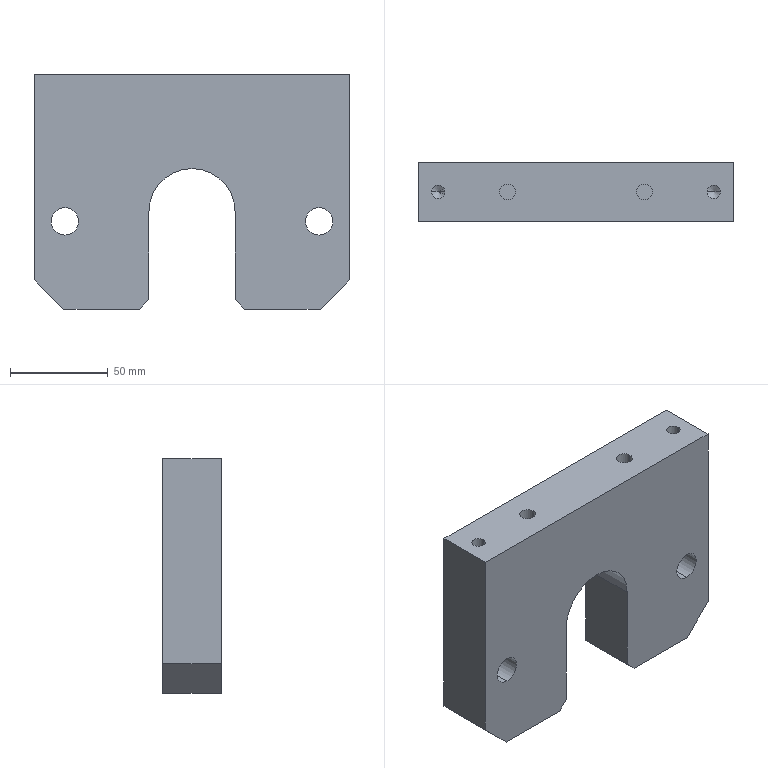Part | SolidWorks | features Chamfer 2, HoleWzd 2, ICE 2, Extrusion 1 | 1 solid | 33 faces | box 161 x 30 x 120 mm | volume 471064 mm3 | plane 15 | cylinder 14 | cone 4 | commonest cylinder face diameters 6.8 x4 8 x4 14 x4 44 x2
STEP:
#1=CARTESIAN_POINT('',(31.,15.,45.));
#2=VERTEX_POINT('',#1);
#3=CARTESIAN_POINT('',(39.,15.,45.));
#4=VERTEX_POINT('',#3);
#5=CARTESIAN_POINT('',(35.,15.,45.));
#6=DIRECTION('',(0.,0.,1.));
#7=DIRECTION('',(1.,0.,0.));
#8=AXIS2_PLACEMENT_3D('',#5,#6,#7);
#9=CIRCLE('',#8,4.);
#10=EDGE_CURVE('',#2,#4,#9,.T.);
#11=ORIENTED_EDGE('',*,*,#10,.F.);
#12=CARTESIAN_POINT('',(31.,15.,60.));
#13=VERTEX_POINT('',#12);
#14=CARTESIAN_POINT('',(31.,15.,45.));
#15=DIRECTION('',(0.,0.,1.));
#16=VECTOR('',#15,1000.);
#17=LINE('',#14,#16);
#18=EDGE_CURVE('',#2,#13,#17,.T.);
#19=ORIENTED_EDGE('',*,*,#18,.T.);
#20=CARTESIAN_POINT('',(39.,15.,60.));
#21=VERTEX_POINT('',#20);
#22=CARTESIAN_POINT('',(35.,15.,60.));
#23=DIRECTION('',(0.,0.,1.));
#24=DIRECTION('',(1.,0.,0.));
#25=AXIS2_PLACEMENT_3D('',#22,#23,#24);
#26=CIRCLE('',#25,4.);
#27=EDGE_CURVE('',#13,#21,#26,.T.);
#28=ORIENTED_EDGE('',*,*,#27,.T.);
#29=CARTESIAN_POINT('',(39.,15.,45.));
#30=DIRECTION('',(0.,0.,1.));
#31=VECTOR('',#30,1000.);
#32=LINE('',#29,#31);
#33=EDGE_CURVE('',#4,#21,#32,.T.);
#34=ORIENTED_EDGE('',*,*,#33,.F.);
#35=EDGE_LOOP('',(#11,#19,#28,#34));
#36=FACE_OUTER_BOUND('',#35,.T.);
#37=CARTESIAN_POINT('',(35.,15.,45.));
#38=DIRECTION('',(0.,0.,1.));
#39=DIRECTION('',(1.,0.,0.));
#40=AXIS2_PLACEMENT_3D('',#37,#38,#39);
#41=CYLINDRICAL_SURFACE('',#40,4.);
#42=ADVANCED_FACE('',(#36),#41,.F.);
#43=CARTESIAN_POINT('',(-39.,15.,45.));
#44=VERTEX_POINT('',#43);
#45=CARTESIAN_POINT('',(-31.,15.,45.));
#46=VERTEX_POINT('',#45);
#47=CARTESIAN_POINT('',(-35.,15.,45.));
#48=DIRECTION('',(0.,0.,1.));
#49=DIRECTION('',(1.,0.,0.));
#50=AXIS2_PLACEMENT_3D('',#47,#48,#49);
#51=CIRCLE('',#50,4.);
#52=EDGE_CURVE('',#44,#46,#51,.T.);
#53=ORIENTED_EDGE('',*,*,#52,.F.);
#54=CARTESIAN_POINT('',(-39.,15.,60.));
#55=VERTEX_POINT('',#54);
#56=CARTESIAN_POINT('',(-39.,15.,45.));
#57=DIRECTION('',(0.,0.,1.));
#58=VECTOR('',#57,1000.);
#59=LINE('',#56,#58);
#60=EDGE_CURVE('',#44,#55,#59,.T.);
#61=ORIENTED_EDGE('',*,*,#60,.T.);
#62=CARTESIAN_POINT('',(-31.,15.,60.));
#63=VERTEX_POINT('',#62);
#64=CARTESIAN_POINT('',(-35.,15.,60.));
#65=DIRECTION('',(0.,0.,1.));
#66=DIRECTION('',(1.,0.,0.));
#67=AXIS2_PLACEMENT_3D('',#64,#65,#66);
#68=CIRCLE('',#67,4.);
#69=EDGE_CURVE('',#55,#63,#68,.T.);
#70=ORIENTED_EDGE('',*,*,#69,.T.);
#71=CARTESIAN_POINT('',(-31.,15.,45.));
#72=DIRECTION('',(0.,0.,1.));
#73=VECTOR('',#72,1000.);
#74=LINE('',#71,#73);
#75=EDGE_CURVE('',#46,#63,#74,.T.);
#76=ORIENTED_EDGE('',*,*,#75,.F.);
#77=EDGE_LOOP('',(#53,#61,#70,#76));
#78=FACE_OUTER_BOUND('',#77,.T.);
#79=CARTESIAN_POINT('',(-35.,15.,45.));
#80=DIRECTION('',(0.,0.,1.));
#81=DIRECTION('',(1.,0.,0.));
#82=AXIS2_PLACEMENT_3D('',#79,#80,#81);
#83=CYLINDRICAL_SURFACE('',#82,4.);
#84=ADVANCED_FACE('',(#78),#83,.F.);
#85=CARTESIAN_POINT('',(67.1,15.,40.25));
#86=VERTEX_POINT('',#85);
#87=CARTESIAN_POINT('',(73.9,15.,40.25));
#88=VERTEX_POINT('',#87);
#89=CARTESIAN_POINT('',(70.5,15.,40.25));
#90=DIRECTION('',(0.,0.,1.));
#91=DIRECTION('',(1.,0.,0.));
#92=AXIS2_PLACEMENT_3D('',#89,#90,#91);
#93=CIRCLE('',#92,3.4);
#94=EDGE_CURVE('',#86,#88,#93,.T.);
#95=ORIENTED_EDGE('',*,*,#94,.F.);
#96=CARTESIAN_POINT('',(67.1,15.,60.));
#97=VERTEX_POINT('',#96);
#98=CARTESIAN_POINT('',(67.1,15.,60.));
#99=DIRECTION('',(0.,0.,1.));
#100=VECTOR('',#99,1000.);
#101=LINE('',#98,#100);
#102=EDGE_CURVE('',#86,#97,#101,.T.);
#103=ORIENTED_EDGE('',*,*,#102,.T.);
#104=CARTESIAN_POINT('',(73.9,15.,60.));
#105=VERTEX_POINT('',#104);
#106=CARTESIAN_POINT('',(70.5,15.,60.));
#107=DIRECTION('',(0.,0.,1.));
#108=DIRECTION('',(1.,0.,0.));
#109=AXIS2_PLACEMENT_3D('',#106,#107,#108);
#110=CIRCLE('',#109,3.4);
#111=EDGE_CURVE('',#97,#105,#110,.T.);
#112=ORIENTED_EDGE('',*,*,#111,.T.);
#113=CARTESIAN_POINT('',(73.9,15.,60.));
#114=DIRECTION('',(0.,0.,1.));
#115=VECTOR('',#114,1000.);
#116=LINE('',#113,#115);
#117=EDGE_CURVE('',#88,#105,#116,.T.);
#118=ORIENTED_EDGE('',*,*,#117,.F.);
#119=EDGE_LOOP('',(#95,#103,#112,#118));
#120=FACE_OUTER_BOUND('',#119,.T.);
#121=CARTESIAN_POINT('',(70.5,15.,60.));
#122=DIRECTION('',(0.,0.,1.));
#123=DIRECTION('',(1.,0.,0.));
#124=AXIS2_PLACEMENT_3D('',#121,#122,#123);
#125=CYLINDRICAL_SURFACE('',#124,3.4);
#126=ADVANCED_FACE('',(#120),#125,.F.);
#127=CARTESIAN_POINT('',(70.5,15.,38.207));
#128=VERTEX_POINT('',#127);
#129=CARTESIAN_POINT('',(73.9,15.,40.25));
#130=DIRECTION('',(0.8572,0.,0.515));
#131=VECTOR('',#130,1000.);
#132=LINE('',#129,#131);
#133=EDGE_CURVE('',#128,#88,#132,.T.);
#134=ORIENTED_EDGE('',*,*,#133,.F.);
#135=CARTESIAN_POINT('',(67.1,15.,40.25));
#136=DIRECTION('',(-0.8572,0.,0.515));
#137=VECTOR('',#136,1000.);
#138=LINE('',#135,#137);
#139=EDGE_CURVE('',#128,#86,#138,.T.);
#140=ORIENTED_EDGE('',*,*,#139,.T.);
#141=ORIENTED_EDGE('',*,*,#94,.T.);
#142=EDGE_LOOP('',(#134,#140,#141));
#143=FACE_OUTER_BOUND('',#142,.T.);
#144=CARTESIAN_POINT('',(70.5,15.,40.25));
#145=DIRECTION('',(0.,0.,1.));
#146=DIRECTION('',(1.,0.,0.));
#147=AXIS2_PLACEMENT_3D('',#144,#145,#146);
#148=CONICAL_SURFACE('',#147,3.4,1.03);
#149=ADVANCED_FACE('',(#143),#148,.F.);
#150=CARTESIAN_POINT('',(-73.9,15.,40.25));
#151=VERTEX_POINT('',#150);
#152=CARTESIAN_POINT('',(-67.1,15.,40.25));
#153=VERTEX_POINT('',#152);
#154=CARTESIAN_POINT('',(-70.5,15.,40.25));
#155=DIRECTION('',(0.,0.,1.));
#156=DIRECTION('',(1.,0.,0.));
#157=AXIS2_PLACEMENT_3D('',#154,#155,#156);
#158=CIRCLE('',#157,3.4);
#159=EDGE_CURVE('',#151,#153,#158,.T.);
#160=ORIENTED_EDGE('',*,*,#159,.F.);
#161=CARTESIAN_POINT('',(-73.9,15.,60.));
#162=VERTEX_POINT('',#161);
#163=CARTESIAN_POINT('',(-73.9,15.,60.));
#164=DIRECTION('',(0.,0.,1.));
#165=VECTOR('',#164,1000.);
#166=LINE('',#163,#165);
#167=EDGE_CURVE('',#151,#162,#166,.T.);
#168=ORIENTED_EDGE('',*,*,#167,.T.);
#169=CARTESIAN_POINT('',(-67.1,15.,60.));
#170=VERTEX_POINT('',#169);
#171=CARTESIAN_POINT('',(-70.5,15.,60.));
#172=DIRECTION('',(0.,0.,1.));
#173=DIRECTION('',(1.,0.,0.));
#174=AXIS2_PLACEMENT_3D('',#171,#172,#173);
#175=CIRCLE('',#174,3.4);
#176=EDGE_CURVE('',#162,#170,#175,.T.);
#177=ORIENTED_EDGE('',*,*,#176,.T.);
#178=CARTESIAN_POINT('',(-67.1,15.,60.));
#179=DIRECTION('',(0.,0.,1.));
#180=VECTOR('',#179,1000.);
#181=LINE('',#178,#180);
#182=EDGE_CURVE('',#153,#170,#181,.T.);
#183=ORIENTED_EDGE('',*,*,#182,.F.);
#184=EDGE_LOOP('',(#160,#168,#177,#183));
#185=FACE_OUTER_BOUND('',#184,.T.);
#186=CARTESIAN_POINT('',(-70.5,15.,60.));
#187=DIRECTION('',(0.,0.,1.));
#188=DIRECTION('',(1.,0.,0.));
#189=AXIS2_PLACEMENT_3D('',#186,#187,#188);
#190=CYLINDRICAL_SURFACE('',#189,3.4);
#191=ADVANCED_FACE('',(#185),#190,.F.);
#192=CARTESIAN_POINT('',(-70.5,15.,38.207));
#193=VERTEX_POINT('',#192);
#194=CARTESIAN_POINT('',(-67.1,15.,40.25));
#195=DIRECTION('',(0.8572,0.,0.515));
#196=VECTOR('',#195,1000.);
#197=LINE('',#194,#196);
#198=EDGE_CURVE('',#193,#153,#197,.T.);
#199=ORIENTED_EDGE('',*,*,#198,.F.);
#200=CARTESIAN_POINT('',(-73.9,15.,40.25));
#201=DIRECTION('',(-0.8572,0.,0.515));
#202=VECTOR('',#201,1000.);
#203=LINE('',#200,#202);
#204=EDGE_CURVE('',#193,#151,#203,.T.);
#205=ORIENTED_EDGE('',*,*,#204,.T.);
#206=ORIENTED_EDGE('',*,*,#159,.T.);
#207=EDGE_LOOP('',(#199,#205,#206));
#208=FACE_OUTER_BOUND('',#207,.T.);
#209=CARTESIAN_POINT('',(-70.5,15.,40.25));
#210=DIRECTION('',(0.,0.,1.));
#211=DIRECTION('',(1.,0.,0.));
#212=AXIS2_PLACEMENT_3D('',#209,#210,#211);
#213=CONICAL_SURFACE('',#212,3.4,1.03);
#214=ADVANCED_FACE('',(#208),#213,.F.);
#215=CARTESIAN_POINT('',(-65.,0.,-22.));
#216=VERTEX_POINT('',#215);
#217=CARTESIAN_POINT('',(-65.,0.,-8.));
#218=VERTEX_POINT('',#217);
#219=CARTESIAN_POINT('',(-65.,0.,-15.));
#220=DIRECTION('',(0.,1.,0.));
#221=DIRECTION('',(0.,0.,1.));
#222=AXIS2_PLACEMENT_3D('',#219,#220,#221);
#223=CIRCLE('',#222,7.);
#224=EDGE_CURVE('',#216,#218,#223,.T.);
#225=ORIENTED_EDGE('',*,*,#224,.F.);
#226=CARTESIAN_POINT('',(-65.,30.,-22.));
#227=VERTEX_POINT('',#226);
#228=CARTESIAN_POINT('',(-65.,30.,-22.));
#229=DIRECTION('',(0.,1.,0.));
#230=VECTOR('',#229,1000.);
#231=LINE('',#228,#230);
#232=EDGE_CURVE('',#216,#227,#231,.T.);
#233=ORIENTED_EDGE('',*,*,#232,.T.);
#234=CARTESIAN_POINT('',(-65.,30.,-8.));
#235=VERTEX_POINT('',#234);
#236=CARTESIAN_POINT('',(-65.,30.,-15.));
#237=DIRECTION('',(0.,1.,0.));
#238=DIRECTION('',(0.,0.,1.));
#239=AXIS2_PLACEMENT_3D('',#236,#237,#238);
#240=CIRCLE('',#239,7.);
#241=EDGE_CURVE('',#227,#235,#240,.T.);
#242=ORIENTED_EDGE('',*,*,#241,.T.);
#243=CARTESIAN_POINT('',(-65.,30.,-8.));
#244=DIRECTION('',(0.,1.,0.));
#245=VECTOR('',#244,1000.);
#246=LINE('',#243,#245);
#247=EDGE_CURVE('',#218,#235,#246,.T.);
#248=ORIENTED_EDGE('',*,*,#247,.F.);
#249=EDGE_LOOP('',(#225,#233,#242,#248));
#250=FACE_OUTER_BOUND('',#249,.T.);
#251=CARTESIAN_POINT('',(-65.,30.,-15.));
#252=DIRECTION('',(0.,1.,0.));
#253=DIRECTION('',(0.,0.,1.));
#254=AXIS2_PLACEMENT_3D('',#251,#252,#253);
#255=CYLINDRICAL_SURFACE('',#254,7.);
#256=ADVANCED_FACE('',(#250),#255,.F.);
#257=CARTESIAN_POINT('',(65.,0.,-22.));
#258=VERTEX_POINT('',#257);
#259=CARTESIAN_POINT('',(65.,0.,-8.));
#260=VERTEX_POINT('',#259);
#261=CARTESIAN_POINT('',(65.,0.,-15.));
#262=DIRECTION('',(0.,1.,0.));
#263=DIRECTION('',(0.,0.,1.));
#264=AXIS2_PLACEMENT_3D('',#261,#262,#263);
#265=CIRCLE('',#264,7.);
#266=EDGE_CURVE('',#258,#260,#265,.T.);
#267=ORIENTED_EDGE('',*,*,#266,.F.);
#268=CARTESIAN_POINT('',(65.,30.,-22.));
#269=VERTEX_POINT('',#268);
#270=CARTESIAN_POINT('',(65.,30.,-22.));
#271=DIRECTION('',(0.,1.,0.));
#272=VECTOR('',#271,1000.);
#273=LINE('',#270,#272);
#274=EDGE_CURVE('',#258,#269,#273,.T.);
#275=ORIENTED_EDGE('',*,*,#274,.T.);
#276=CARTESIAN_POINT('',(65.,30.,-8.));
#277=VERTEX_POINT('',#276);
#278=CARTESIAN_POINT('',(65.,30.,-15.));
#279=DIRECTION('',(0.,1.,0.));
#280=DIRECTION('',(0.,0.,1.));
#281=AXIS2_PLACEMENT_3D('',#278,#279,#280);
#282=CIRCLE('',#281,7.);
#283=EDGE_CURVE('',#269,#277,#282,.T.);
#284=ORIENTED_EDGE('',*,*,#283,.T.);
#285=CARTESIAN_POINT('',(65.,30.,-8.));
#286=DIRECTION('',(0.,1.,0.));
#287=VECTOR('',#286,1000.);
#288=LINE('',#285,#287);
#289=EDGE_CURVE('',#260,#277,#288,.T.);
#290=ORIENTED_EDGE('',*,*,#289,.F.);
#291=EDGE_LOOP('',(#267,#275,#284,#290));
#292=FACE_OUTER_BOUND('',#291,.T.);
#293=CARTESIAN_POINT('',(65.,30.,-15.));
#294=DIRECTION('',(0.,1.,0.));
#295=DIRECTION('',(0.,0.,1.));
#296=AXIS2_PLACEMENT_3D('',#293,#294,#295);
#297=CYLINDRICAL_SURFACE('',#296,7.);
#298=ADVANCED_FACE('',(#292),#297,.F.);
#299=CARTESIAN_POINT('',(0.,0.,12.));
#300=VERTEX_POINT('',#299);
#301=CARTESIAN_POINT('',(22.,0.,-10.));
#302=VERTEX_POINT('',#301);
#303=CARTESIAN_POINT('',(0.,0.,-10.));
#304=DIRECTION('',(0.,1.,0.));
#305=DIRECTION('',(0.,0.,1.));
#306=AXIS2_PLACEMENT_3D('',#303,#304,#305);
#307=CIRCLE('',#306,22.);
#308=EDGE_CURVE('',#300,#302,#307,.T.);
#309=ORIENTED_EDGE('',*,*,#308,.F.);
#310=CARTESIAN_POINT('',(0.,30.,12.));
#311=VERTEX_POINT('',#310);
#312=CARTESIAN_POINT('',(0.,0.,12.));
#313=DIRECTION('',(0.,1.,0.));
#314=VECTOR('',#313,1000.);
#315=LINE('',#312,#314);
#316=EDGE_CURVE('',#300,#311,#315,.T.);
#317=ORIENTED_EDGE('',*,*,#316,.T.);
#318=CARTESIAN_POINT('',(22.,30.,-10.));
#319=VERTEX_POINT('',#318);
#320=CARTESIAN_POINT('',(0.,30.,-10.));
#321=DIRECTION('',(0.,1.,0.));
#322=DIRECTION('',(0.,0.,1.));
#323=AXIS2_PLACEMENT_3D('',#320,#321,#322);
#324=CIRCLE('',#323,22.);
#325=EDGE_CURVE('',#311,#319,#324,.T.);
#326=ORIENTED_EDGE('',*,*,#325,.T.);
#327=CARTESIAN_POINT('',(22.,0.,-10.));
#328=DIRECTION('',(0.,1.,0.));
#329=VECTOR('',#328,1000.);
#330=LINE('',#327,#329);
#331=EDGE_CURVE('',#302,#319,#330,.T.);
#332=ORIENTED_EDGE('',*,*,#331,.F.);
#333=EDGE_LOOP('',(#309,#317,#326,#332));
#334=FACE_OUTER_BOUND('',#333,.T.);
#335=CARTESIAN_POINT('',(0.,0.,-10.));
#336=DIRECTION('',(0.,1.,0.));
#337=DIRECTION('',(0.,0.,1.));
#338=AXIS2_PLACEMENT_3D('',#335,#336,#337);
#339=CYLINDRICAL_SURFACE('',#338,22.);
#340=ADVANCED_FACE('',(#334),#339,.F.);
#341=CARTESIAN_POINT('',(-27.,30.,-60.));
#342=VERTEX_POINT('',#341);
#343=CARTESIAN_POINT('',(-65.5,30.,-60.));
#344=VERTEX_POINT('',#343);
#345=CARTESIAN_POINT('',(80.5,30.,-60.));
#346=DIRECTION('',(-1.,0.,0.));
#347=VECTOR('',#346,1000.);
#348=LINE('',#345,#347);
#349=EDGE_CURVE('',#342,#344,#348,.T.);
#350=ORIENTED_EDGE('',*,*,#349,.F.);
#351=CARTESIAN_POINT('',(-27.,0.,-60.));
#352=VERTEX_POINT('',#351);
#353=CARTESIAN_POINT('',(-27.,30.,-60.));
#354=DIRECTION('',(0.,-1.,0.));
#355=VECTOR('',#354,1000.);
#356=LINE('',#353,#355);
#357=EDGE_CURVE('',#342,#352,#356,.T.);
#358=ORIENTED_EDGE('',*,*,#357,.T.);
#359=CARTESIAN_POINT('',(-65.5,0.,-60.));
#360=VERTEX_POINT('',#359);
#361=CARTESIAN_POINT('',(80.5,0.,-60.));
#362=DIRECTION('',(-1.,0.,0.));
#363=VECTOR('',#362,1000.);
#364=LINE('',#361,#363);
#365=EDGE_CURVE('',#352,#360,#364,.T.);
#366=ORIENTED_EDGE('',*,*,#365,.T.);
#367=CARTESIAN_POINT('',(-65.5,30.,-60.));
#368=DIRECTION('',(0.,1.,0.));
#369=VECTOR('',#368,1000.);
#370=LINE('',#367,#369);
#371=EDGE_CURVE('',#360,#344,#370,.T.);
#372=ORIENTED_EDGE('',*,*,#371,.T.);
#373=EDGE_LOOP('',(#350,#358,#366,#372));
#374=FACE_OUTER_BOUND('',#373,.T.);
#375=CARTESIAN_POINT('',(80.5,30.,-60.));
#376=DIRECTION('',(0.,0.,1.));
#377=DIRECTION('',(1.,0.,0.));
#378=AXIS2_PLACEMENT_3D('',#375,#376,#377);
#379=PLANE('',#378);
#380=ADVANCED_FACE('',(#374),#379,.F.);
#381=CARTESIAN_POINT('',(-80.5,30.,-45.));
#382=VERTEX_POINT('',#381);
#383=CARTESIAN_POINT('',(-80.5,30.,60.));
#384=VERTEX_POINT('',#383);
#385=CARTESIAN_POINT('',(-80.5,30.,60.));
#386=DIRECTION('',(0.,0.,1.));
#387=VECTOR('',#386,1000.);
#388=LINE('',#385,#387);
#389=EDGE_CURVE('',#382,#384,#388,.T.);
#390=ORIENTED_EDGE('',*,*,#389,.F.);
#391=CARTESIAN_POINT('',(-80.5,0.,-45.));
#392=VERTEX_POINT('',#391);
#393=CARTESIAN_POINT('',(-80.5,30.,-45.));
#394=DIRECTION('',(0.,-1.,0.));
#395=VECTOR('',#394,1000.);
#396=LINE('',#393,#395);
#397=EDGE_CURVE('',#382,#392,#396,.T.);
#398=ORIENTED_EDGE('',*,*,#397,.T.);
#399=CARTESIAN_POINT('',(-80.5,0.,60.));
#400=VERTEX_POINT('',#399);
#401=CARTESIAN_POINT('',(-80.5,0.,60.));
#402=DIRECTION('',(0.,0.,1.));
#403=VECTOR('',#402,1000.);
#404=LINE('',#401,#403);
#405=EDGE_CURVE('',#392,#400,#404,.T.);
#406=ORIENTED_EDGE('',*,*,#405,.T.);
#407=CARTESIAN_POINT('',(-80.5,30.,60.));
#408=DIRECTION('',(0.,-1.,0.));
#409=VECTOR('',#408,1000.);
#410=LINE('',#407,#409);
#411=EDGE_CURVE('',#384,#400,#410,.T.);
#412=ORIENTED_EDGE('',*,*,#411,.F.);
#413=EDGE_LOOP('',(#390,#398,#406,#412));
#414=FACE_OUTER_BOUND('',#413,.T.);
#415=CARTESIAN_POINT('',(-80.5,30.,60.));
#416=DIRECTION('',(1.,0.,0.));
#417=DIRECTION('',(0.,0.,-1.));
#418=AXIS2_PLACEMENT_3D('',#415,#416,#417);
#419=PLANE('',#418);
#420=ADVANCED_FACE('',(#414),#419,.F.);
#421=CARTESIAN_POINT('',(35.,15.,60.));
#422=DIRECTION('',(0.,0.,1.));
#423=DIRECTION('',(1.,0.,0.));
#424=AXIS2_PLACEMENT_3D('',#421,#422,#423);
#425=CIRCLE('',#424,4.);
#426=EDGE_CURVE('',#21,#13,#425,.T.);
#427=ORIENTED_EDGE('',*,*,#426,.F.);
#428=ORIENTED_EDGE('',*,*,#27,.F.);
#429=EDGE_LOOP('',(#427,#428));
#430=FACE_BOUND('',#429,.T.);
#431=CARTESIAN_POINT('',(-35.,15.,60.));
#432=DIRECTION('',(0.,0.,1.));
#433=DIRECTION('',(1.,0.,0.));
#434=AXIS2_PLACEMENT_3D('',#431,#432,#433);
#435=CIRCLE('',#434,4.);
#436=EDGE_CURVE('',#63,#55,#435,.T.);
#437=ORIENTED_EDGE('',*,*,#436,.F.);
#438=ORIENTED_EDGE('',*,*,#69,.F.);
#439=EDGE_LOOP('',(#437,#438));
#440=FACE_BOUND('',#439,.T.);
#441=CARTESIAN_POINT('',(70.5,15.,60.));
#442=DIRECTION('',(0.,0.,1.));
#443=DIRECTION('',(1.,0.,0.));
#444=AXIS2_PLACEMENT_3D('',#441,#442,#443);
#445=CIRCLE('',#444,3.4);
#446=EDGE_CURVE('',#105,#97,#445,.T.);
#447=ORIENTED_EDGE('',*,*,#446,.F.);
#448=ORIENTED_EDGE('',*,*,#111,.F.);
#449=EDGE_LOOP('',(#447,#448));
#450=FACE_BOUND('',#449,.T.);
#451=CARTESIAN_POINT('',(-70.5,15.,60.));
#452=DIRECTION('',(0.,0.,1.));
#453=DIRECTION('',(1.,0.,0.));
#454=AXIS2_PLACEMENT_3D('',#451,#452,#453);
#455=CIRCLE('',#454,3.4);
#456=EDGE_CURVE('',#170,#162,#455,.T.);
#457=ORIENTED_EDGE('',*,*,#456,.F.);
#458=ORIENTED_EDGE('',*,*,#176,.F.);
#459=EDGE_LOOP('',(#457,#458));
#460=FACE_BOUND('',#459,.T.);
#461=CARTESIAN_POINT('',(80.5,0.,60.));
#462=VERTEX_POINT('',#461);
#463=CARTESIAN_POINT('',(80.5,0.,60.));
#464=DIRECTION('',(1.,0.,0.));
#465=VECTOR('',#464,1000.);
#466=LINE('',#463,#465);
#467=EDGE_CURVE('',#400,#462,#466,.T.);
#468=ORIENTED_EDGE('',*,*,#467,.T.);
#469=CARTESIAN_POINT('',(80.5,30.,60.));
#470=VERTEX_POINT('',#469);
#471=CARTESIAN_POINT('',(80.5,30.,60.));
#472=DIRECTION('',(0.,-1.,0.));
#473=VECTOR('',#472,1000.);
#474=LINE('',#471,#473);
#475=EDGE_CURVE('',#470,#462,#474,.T.);
#476=ORIENTED_EDGE('',*,*,#475,.F.);
#477=CARTESIAN_POINT('',(80.5,30.,60.));
#478=DIRECTION('',(1.,0.,0.));
#479=VECTOR('',#478,1000.);
#480=LINE('',#477,#479);
#481=EDGE_CURVE('',#384,#470,#480,.T.);
#482=ORIENTED_EDGE('',*,*,#481,.F.);
#483=ORIENTED_EDGE('',*,*,#411,.T.);
#484=EDGE_LOOP('',(#468,#476,#482,#483));
#485=FACE_OUTER_BOUND('',#484,.T.);
#486=CARTESIAN_POINT('',(80.5,30.,60.));
#487=DIRECTION('',(0.,0.,-1.));
#488=DIRECTION('',(-1.,0.,0.));
#489=AXIS2_PLACEMENT_3D('',#486,#487,#488);
#490=PLANE('',#489);
#491=ADVANCED_FACE('',(#430,#440,#450,#460,#485),#490,.F.);
#492=CARTESIAN_POINT('',(80.5,0.,-45.));
#493=VERTEX_POINT('',#492);
#494=CARTESIAN_POINT('',(80.5,0.,60.));
#495=DIRECTION('',(0.,0.,-1.));
#496=VECTOR('',#495,1000.);
#497=LINE('',#494,#496);
#498=EDGE_CURVE('',#462,#493,#497,.T.);
#499=ORIENTED_EDGE('',*,*,#498,.T.);
#500=CARTESIAN_POINT('',(80.5,30.,-45.));
#501=VERTEX_POINT('',#500);
#502=CARTESIAN_POINT('',(80.5,30.,-45.));
#503=DIRECTION('',(0.,1.,0.));
#504=VECTOR('',#503,1000.);
#505=LINE('',#502,#504);
#506=EDGE_CURVE('',#493,#501,#505,.T.);
#507=ORIENTED_EDGE('',*,*,#506,.T.);
#508=CARTESIAN_POINT('',(80.5,30.,60.));
#509=DIRECTION('',(0.,0.,-1.));
#510=VECTOR('',#509,1000.);
#511=LINE('',#508,#510);
#512=EDGE_CURVE('',#470,#501,#511,.T.);
#513=ORIENTED_EDGE('',*,*,#512,.F.);
#514=ORIENTED_EDGE('',*,*,#475,.T.);
#515=EDGE_LOOP('',(#499,#507,#513,#514));
#516=FACE_OUTER_BOUND('',#515,.T.);
#517=CARTESIAN_POINT('',(80.5,30.,60.));
#518=DIRECTION('',(-1.,0.,0.));
#519=DIRECTION('',(0.,0.,1.));
#520=AXIS2_PLACEMENT_3D('',#517,#518,#519);
#521=PLANE('',#520);
#522=ADVANCED_FACE('',(#516),#521,.F.);
#523=CARTESIAN_POINT('',(65.5,0.,-60.));
#524=VERTEX_POINT('',#523);
#525=CARTESIAN_POINT('',(27.,0.,-60.));
#526=VERTEX_POINT('',#525);
#527=CARTESIAN_POINT('',(80.5,0.,-60.));
#528=DIRECTION('',(-1.,0.,0.));
#529=VECTOR('',#528,1000.);
#530=LINE('',#527,#529);
#531=EDGE_CURVE('',#524,#526,#530,.T.);
#532=ORIENTED_EDGE('',*,*,#531,.T.);
#533=CARTESIAN_POINT('',(27.,30.,-60.));
#534=VERTEX_POINT('',#533);
#535=CARTESIAN_POINT('',(27.,30.,-60.));
#536=DIRECTION('',(0.,1.,0.));
#537=VECTOR('',#536,1000.);
#538=LINE('',#535,#537);
#539=EDGE_CURVE('',#526,#534,#538,.T.);
#540=ORIENTED_EDGE('',*,*,#539,.T.);
#541=CARTESIAN_POINT('',(65.5,30.,-60.));
#542=VERTEX_POINT('',#541);
#543=CARTESIAN_POINT('',(80.5,30.,-60.));
#544=DIRECTION('',(-1.,0.,0.));
#545=VECTOR('',#544,1000.);
#546=LINE('',#543,#545);
#547=EDGE_CURVE('',#542,#534,#546,.T.);
#548=ORIENTED_EDGE('',*,*,#547,.F.);
#549=CARTESIAN_POINT('',(65.5,30.,-60.));
#550=DIRECTION('',(0.,-1.,0.));
#551=VECTOR('',#550,1000.);
#552=LINE('',#549,#551);
#553=EDGE_CURVE('',#542,#524,#552,.T.);
#554=ORIENTED_EDGE('',*,*,#553,.T.);
#555=EDGE_LOOP('',(#532,#540,#548,#554));
#556=FACE_OUTER_BOUND('',#555,.T.);
#557=CARTESIAN_POINT('',(80.5,30.,-60.));
#558=DIRECTION('',(0.,0.,1.));
#559=DIRECTION('',(1.,0.,0.));
#560=AXIS2_PLACEMENT_3D('',#557,#558,#559);
#561=PLANE('',#560);
#562=ADVANCED_FACE('',(#556),#561,.F.);
#563=CARTESIAN_POINT('',(-65.,30.,-15.));
#564=DIRECTION('',(0.,1.,0.));
#565=DIRECTION('',(0.,0.,1.));
#566=AXIS2_PLACEMENT_3D('',#563,#564,#565);
#567=CIRCLE('',#566,7.);
#568=EDGE_CURVE('',#235,#227,#567,.T.);
#569=ORIENTED_EDGE('',*,*,#568,.F.);
#570=ORIENTED_EDGE('',*,*,#241,.F.);
#571=EDGE_LOOP('',(#569,#570));
#572=FACE_BOUND('',#571,.T.);
#573=CARTESIAN_POINT('',(65.,30.,-15.));
#574=DIRECTION('',(0.,1.,0.));
#575=DIRECTION('',(0.,0.,1.));
#576=AXIS2_PLACEMENT_3D('',#573,#574,#575);
#577=CIRCLE('',#576,7.);
#578=EDGE_CURVE('',#277,#269,#577,.T.);
#579=ORIENTED_EDGE('',*,*,#578,.F.);
#580=ORIENTED_EDGE('',*,*,#283,.F.);
#581=EDGE_LOOP('',(#579,#580));
#582=FACE_BOUND('',#581,.T.);
#583=ORIENTED_EDGE('',*,*,#547,.T.);
#584=CARTESIAN_POINT('',(22.,30.,-55.));
#585=VERTEX_POINT('',#584);
#586=CARTESIAN_POINT('',(-26.75,30.,-6.25));
#587=DIRECTION('',(-0.7071,0.,0.7071));
#588=VECTOR('',#587,1000.);
#589=LINE('',#586,#588);
#590=EDGE_CURVE('',#534,#585,#589,.T.);
#591=ORIENTED_EDGE('',*,*,#590,.T.);
#592=CARTESIAN_POINT('',(22.,30.,-60.));
#593=DIRECTION('',(0.,0.,-1.));
#594=VECTOR('',#593,1000.);
#595=LINE('',#592,#594);
#596=EDGE_CURVE('',#319,#585,#595,.T.);
#597=ORIENTED_EDGE('',*,*,#596,.F.);
#598=ORIENTED_EDGE('',*,*,#325,.F.);
#599=CARTESIAN_POINT('',(-22.,30.,-10.));
#600=VERTEX_POINT('',#599);
#601=CARTESIAN_POINT('',(0.,30.,-10.));
#602=DIRECTION('',(0.,1.,0.));
#603=DIRECTION('',(0.,0.,1.));
#604=AXIS2_PLACEMENT_3D('',#601,#602,#603);
#605=CIRCLE('',#604,22.);
#606=EDGE_CURVE('',#600,#311,#605,.T.);
#607=ORIENTED_EDGE('',*,*,#606,.F.);
#608=CARTESIAN_POINT('',(-22.,30.,-55.));
#609=VERTEX_POINT('',#608);
#610=CARTESIAN_POINT('',(-22.,30.,-10.));
#611=DIRECTION('',(0.,0.,1.));
#612=VECTOR('',#611,1000.);
#613=LINE('',#610,#612);
#614=EDGE_CURVE('',#609,#600,#613,.T.);
#615=ORIENTED_EDGE('',*,*,#614,.F.);
#616=CARTESIAN_POINT('',(-53.75,30.,-86.75));
#617=DIRECTION('',(-0.7071,0.,-0.7071));
#618=VECTOR('',#617,1000.);
#619=LINE('',#616,#618);
#620=EDGE_CURVE('',#609,#342,#619,.T.);
#621=ORIENTED_EDGE('',*,*,#620,.T.);
#622=ORIENTED_EDGE('',*,*,#349,.T.);
#623=CARTESIAN_POINT('',(-73.,30.,-52.5));
#624=DIRECTION('',(-0.7071,0.,0.7071));
#625=VECTOR('',#624,1000.);
#626=LINE('',#623,#625);
#627=EDGE_CURVE('',#344,#382,#626,.T.);
#628=ORIENTED_EDGE('',*,*,#627,.T.);
#629=ORIENTED_EDGE('',*,*,#389,.T.);
#630=ORIENTED_EDGE('',*,*,#481,.T.);
#631=ORIENTED_EDGE('',*,*,#512,.T.);
#632=CARTESIAN_POINT('',(-7.5,30.,-133.));
#633=DIRECTION('',(-0.7071,0.,-0.7071));
#634=VECTOR('',#633,1000.);
#635=LINE('',#632,#634);
#636=EDGE_CURVE('',#501,#542,#635,.T.);
#637=ORIENTED_EDGE('',*,*,#636,.T.);
#638=EDGE_LOOP('',(#583,#591,#597,#598,#607,#615,#621,#622,#628,#629,#630,#631,#637));
#639=FACE_OUTER_BOUND('',#638,.T.);
#640=CARTESIAN_POINT('',(-80.5,30.,-60.));
#641=DIRECTION('',(0.,1.,0.));
#642=DIRECTION('',(0.,0.,1.));
#643=AXIS2_PLACEMENT_3D('',#640,#641,#642);
#644=PLANE('',#643);
#645=ADVANCED_FACE('',(#572,#582,#639),#644,.T.);
#646=CARTESIAN_POINT('',(-65.,0.,-15.));
#647=DIRECTION('',(0.,1.,0.));
#648=DIRECTION('',(0.,0.,1.));
#649=AXIS2_PLACEMENT_3D('',#646,#647,#648);
#650=CIRCLE('',#649,7.);
#651=EDGE_CURVE('',#218,#216,#650,.T.);
#652=ORIENTED_EDGE('',*,*,#651,.T.);
#653=ORIENTED_EDGE('',*,*,#224,.T.);
#654=EDGE_LOOP('',(#652,#653));
#655=FACE_BOUND('',#654,.T.);
#656=CARTESIAN_POINT('',(65.,0.,-15.));
#657=DIRECTION('',(0.,1.,0.));
#658=DIRECTION('',(0.,0.,1.));
#659=AXIS2_PLACEMENT_3D('',#656,#657,#658);
#660=CIRCLE('',#659,7.);
#661=EDGE_CURVE('',#260,#258,#660,.T.);
#662=ORIENTED_EDGE('',*,*,#661,.T.);
#663=ORIENTED_EDGE('',*,*,#266,.T.);
#664=EDGE_LOOP('',(#662,#663));
#665=FACE_BOUND('',#664,.T.);
#666=CARTESIAN_POINT('',(22.,0.,-55.));
#667=VERTEX_POINT('',#666);
#668=CARTESIAN_POINT('',(22.,0.,-60.));
#669=DIRECTION('',(0.,0.,-1.));
#670=VECTOR('',#669,1000.);
#671=LINE('',#668,#670);
#672=EDGE_CURVE('',#302,#667,#671,.T.);
#673=ORIENTED_EDGE('',*,*,#672,.T.);
#674=CARTESIAN_POINT('',(27.,0.,-60.));
#675=DIRECTION('',(0.7071,0.,-0.7071));
#676=VECTOR('',#675,1000.);
#677=LINE('',#674,#676);
#678=EDGE_CURVE('',#667,#526,#677,.T.);
#679=ORIENTED_EDGE('',*,*,#678,.T.);
#680=ORIENTED_EDGE('',*,*,#531,.F.);
#681=CARTESIAN_POINT('',(65.5,0.,-60.));
#682=DIRECTION('',(0.7071,0.,0.7071));
#683=VECTOR('',#682,1000.);
#684=LINE('',#681,#683);
#685=EDGE_CURVE('',#524,#493,#684,.T.);
#686=ORIENTED_EDGE('',*,*,#685,.T.);
#687=ORIENTED_EDGE('',*,*,#498,.F.);
#688=ORIENTED_EDGE('',*,*,#467,.F.);
#689=ORIENTED_EDGE('',*,*,#405,.F.);
#690=CARTESIAN_POINT('',(-80.5,0.,-45.));
#691=DIRECTION('',(0.7071,0.,-0.7071));
#692=VECTOR('',#691,1000.);
#693=LINE('',#690,#692);
#694=EDGE_CURVE('',#392,#360,#693,.T.);
#695=ORIENTED_EDGE('',*,*,#694,.T.);
#696=ORIENTED_EDGE('',*,*,#365,.F.);
#697=CARTESIAN_POINT('',(-22.,0.,-55.));
#698=VERTEX_POINT('',#697);
#699=CARTESIAN_POINT('',(-22.,0.,-55.));
#700=DIRECTION('',(0.7071,0.,0.7071));
#701=VECTOR('',#700,1000.);
#702=LINE('',#699,#701);
#703=EDGE_CURVE('',#352,#698,#702,.T.);
#704=ORIENTED_EDGE('',*,*,#703,.T.);
#705=CARTESIAN_POINT('',(-22.,0.,-10.));
#706=VERTEX_POINT('',#705);
#707=CARTESIAN_POINT('',(-22.,0.,-10.));
#708=DIRECTION('',(0.,0.,1.));
#709=VECTOR('',#708,1000.);
#710=LINE('',#707,#709);
#711=EDGE_CURVE('',#698,#706,#710,.T.);
#712=ORIENTED_EDGE('',*,*,#711,.T.);
#713=CARTESIAN_POINT('',(0.,0.,-10.));
#714=DIRECTION('',(0.,1.,0.));
#715=DIRECTION('',(0.,0.,1.));
#716=AXIS2_PLACEMENT_3D('',#713,#714,#715);
#717=CIRCLE('',#716,22.);
#718=EDGE_CURVE('',#706,#300,#717,.T.);
#719=ORIENTED_EDGE('',*,*,#718,.T.);
#720=ORIENTED_EDGE('',*,*,#308,.T.);
#721=EDGE_LOOP('',(#673,#679,#680,#686,#687,#688,#689,#695,#696,#704,#712,#719,#720));
#722=FACE_OUTER_BOUND('',#721,.T.);
#723=CARTESIAN_POINT('',(-80.5,0.,-60.));
#724=DIRECTION('',(0.,1.,0.));
#725=DIRECTION('',(0.,0.,1.));
#726=AXIS2_PLACEMENT_3D('',#723,#724,#725);
#727=PLANE('',#726);
#728=ADVANCED_FACE('',(#655,#665,#722),#727,.F.);
#729=ORIENTED_EDGE('',*,*,#316,.F.);
#730=ORIENTED_EDGE('',*,*,#718,.F.);
#731=CARTESIAN_POINT('',(-22.,0.,-10.));
#732=DIRECTION('',(0.,1.,0.));
#733=VECTOR('',#732,1000.);
#734=LINE('',#731,#733);
#735=EDGE_CURVE('',#706,#600,#734,.T.);
#736=ORIENTED_EDGE('',*,*,#735,.T.);
#737=ORIENTED_EDGE('',*,*,#606,.T.);
#738=EDGE_LOOP('',(#729,#730,#736,#737));
#739=FACE_OUTER_BOUND('',#738,.T.);
#740=CARTESIAN_POINT('',(0.,0.,-10.));
#741=DIRECTION('',(0.,1.,0.));
#742=DIRECTION('',(0.,0.,1.));
#743=AXIS2_PLACEMENT_3D('',#740,#741,#742);
#744=CYLINDRICAL_SURFACE('',#743,22.);
#745=ADVANCED_FACE('',(#739),#744,.F.);
#746=ORIENTED_EDGE('',*,*,#711,.F.);
#747=CARTESIAN_POINT('',(-22.,0.,-55.));
#748=DIRECTION('',(0.,1.,0.));
#749=VECTOR('',#748,1000.);
#750=LINE('',#747,#749);
#751=EDGE_CURVE('',#698,#609,#750,.T.);
#752=ORIENTED_EDGE('',*,*,#751,.T.);
#753=ORIENTED_EDGE('',*,*,#614,.T.);
#754=ORIENTED_EDGE('',*,*,#735,.F.);
#755=EDGE_LOOP('',(#746,#752,#753,#754));
#756=FACE_OUTER_BOUND('',#755,.T.);
#757=CARTESIAN_POINT('',(-22.,0.,-10.));
#758=DIRECTION('',(-1.,0.,0.));
#759=DIRECTION('',(0.,0.,1.));
#760=AXIS2_PLACEMENT_3D('',#757,#758,#759);
#761=PLANE('',#760);
#762=ADVANCED_FACE('',(#756),#761,.F.);
#763=ORIENTED_EDGE('',*,*,#596,.T.);
#764=CARTESIAN_POINT('',(22.,0.,-55.));
#765=DIRECTION('',(0.,-1.,0.));
#766=VECTOR('',#765,1000.);
#767=LINE('',#764,#766);
#768=EDGE_CURVE('',#585,#667,#767,.T.);
#769=ORIENTED_EDGE('',*,*,#768,.T.);
#770=ORIENTED_EDGE('',*,*,#672,.F.);
#771=ORIENTED_EDGE('',*,*,#331,.T.);
#772=EDGE_LOOP('',(#763,#769,#770,#771));
#773=FACE_OUTER_BOUND('',#772,.T.);
#774=CARTESIAN_POINT('',(22.,0.,-60.));
#775=DIRECTION('',(1.,0.,0.));
#776=DIRECTION('',(0.,0.,-1.));
#777=AXIS2_PLACEMENT_3D('',#774,#775,#776);
#778=PLANE('',#777);
#779=ADVANCED_FACE('',(#773),#778,.F.);
#780=ORIENTED_EDGE('',*,*,#274,.F.);
#781=ORIENTED_EDGE('',*,*,#661,.F.);
#782=ORIENTED_EDGE('',*,*,#289,.T.);
#783=ORIENTED_EDGE('',*,*,#578,.T.);
#784=EDGE_LOOP('',(#780,#781,#782,#783));
#785=FACE_OUTER_BOUND('',#784,.T.);
#786=CARTESIAN_POINT('',(65.,30.,-15.));
#787=DIRECTION('',(0.,1.,0.));
#788=DIRECTION('',(0.,0.,1.));
#789=AXIS2_PLACEMENT_3D('',#786,#787,#788);
#790=CYLINDRICAL_SURFACE('',#789,7.);
#791=ADVANCED_FACE('',(#785),#790,.F.);
#792=ORIENTED_EDGE('',*,*,#232,.F.);
#793=ORIENTED_EDGE('',*,*,#651,.F.);
#794=ORIENTED_EDGE('',*,*,#247,.T.);
#795=ORIENTED_EDGE('',*,*,#568,.T.);
#796=EDGE_LOOP('',(#792,#793,#794,#795));
#797=FACE_OUTER_BOUND('',#796,.T.);
#798=CARTESIAN_POINT('',(-65.,30.,-15.));
#799=DIRECTION('',(0.,1.,0.));
#800=DIRECTION('',(0.,0.,1.));
#801=AXIS2_PLACEMENT_3D('',#798,#799,#800);
#802=CYLINDRICAL_SURFACE('',#801,7.);
#803=ADVANCED_FACE('',(#797),#802,.F.);
#804=ORIENTED_EDGE('',*,*,#204,.F.);
#805=ORIENTED_EDGE('',*,*,#198,.T.);
#806=CARTESIAN_POINT('',(-70.5,15.,40.25));
#807=DIRECTION('',(0.,0.,1.));
#808=DIRECTION('',(1.,0.,0.));
#809=AXIS2_PLACEMENT_3D('',#806,#807,#808);
#810=CIRCLE('',#809,3.4);
#811=EDGE_CURVE('',#153,#151,#810,.T.);
#812=ORIENTED_EDGE('',*,*,#811,.T.);
#813=EDGE_LOOP('',(#804,#805,#812));
#814=FACE_OUTER_BOUND('',#813,.T.);
#815=CARTESIAN_POINT('',(-70.5,15.,40.25));
#816=DIRECTION('',(0.,0.,1.));
#817=DIRECTION('',(1.,0.,0.));
#818=AXIS2_PLACEMENT_3D('',#815,#816,#817);
#819=CONICAL_SURFACE('',#818,3.4,1.03);
#820=ADVANCED_FACE('',(#814),#819,.F.);
#821=ORIENTED_EDGE('',*,*,#167,.F.);
#822=ORIENTED_EDGE('',*,*,#811,.F.);
#823=ORIENTED_EDGE('',*,*,#182,.T.);
#824=ORIENTED_EDGE('',*,*,#456,.T.);
#825=EDGE_LOOP('',(#821,#822,#823,#824));
#826=FACE_OUTER_BOUND('',#825,.T.);
#827=CARTESIAN_POINT('',(-70.5,15.,60.));
#828=DIRECTION('',(0.,0.,1.));
#829=DIRECTION('',(1.,0.,0.));
#830=AXIS2_PLACEMENT_3D('',#827,#828,#829);
#831=CYLINDRICAL_SURFACE('',#830,3.4);
#832=ADVANCED_FACE('',(#826),#831,.F.);
#833=ORIENTED_EDGE('',*,*,#139,.F.);
#834=ORIENTED_EDGE('',*,*,#133,.T.);
#835=CARTESIAN_POINT('',(70.5,15.,40.25));
#836=DIRECTION('',(0.,0.,1.));
#837=DIRECTION('',(1.,0.,0.));
#838=AXIS2_PLACEMENT_3D('',#835,#836,#837);
#839=CIRCLE('',#838,3.4);
#840=EDGE_CURVE('',#88,#86,#839,.T.);
#841=ORIENTED_EDGE('',*,*,#840,.T.);
#842=EDGE_LOOP('',(#833,#834,#841));
#843=FACE_OUTER_BOUND('',#842,.T.);
#844=CARTESIAN_POINT('',(70.5,15.,40.25));
#845=DIRECTION('',(0.,0.,1.));
#846=DIRECTION('',(1.,0.,0.));
#847=AXIS2_PLACEMENT_3D('',#844,#845,#846);
#848=CONICAL_SURFACE('',#847,3.4,1.03);
#849=ADVANCED_FACE('',(#843),#848,.F.);
#850=ORIENTED_EDGE('',*,*,#102,.F.);
#851=ORIENTED_EDGE('',*,*,#840,.F.);
#852=ORIENTED_EDGE('',*,*,#117,.T.);
#853=ORIENTED_EDGE('',*,*,#446,.T.);
#854=EDGE_LOOP('',(#850,#851,#852,#853));
#855=FACE_OUTER_BOUND('',#854,.T.);
#856=CARTESIAN_POINT('',(70.5,15.,60.));
#857=DIRECTION('',(0.,0.,1.));
#858=DIRECTION('',(1.,0.,0.));
#859=AXIS2_PLACEMENT_3D('',#856,#857,#858);
#860=CYLINDRICAL_SURFACE('',#859,3.4);
#861=ADVANCED_FACE('',(#855),#860,.F.);
#862=ORIENTED_EDGE('',*,*,#60,.F.);
#863=CARTESIAN_POINT('',(-35.,15.,45.));
#864=DIRECTION('',(0.,0.,1.));
#865=DIRECTION('',(1.,0.,0.));
#866=AXIS2_PLACEMENT_3D('',#863,#864,#865);
#867=CIRCLE('',#866,4.);
#868=EDGE_CURVE('',#46,#44,#867,.T.);
#869=ORIENTED_EDGE('',*,*,#868,.F.);
#870=ORIENTED_EDGE('',*,*,#75,.T.);
#871=ORIENTED_EDGE('',*,*,#436,.T.);
#872=EDGE_LOOP('',(#862,#869,#870,#871));
#873=FACE_OUTER_BOUND('',#872,.T.);
#874=CARTESIAN_POINT('',(-35.,15.,45.));
#875=DIRECTION('',(0.,0.,1.));
#876=DIRECTION('',(1.,0.,0.));
#877=AXIS2_PLACEMENT_3D('',#874,#875,#876);
#878=CYLINDRICAL_SURFACE('',#877,4.);
#879=ADVANCED_FACE('',(#873),#878,.F.);
#880=ORIENTED_EDGE('',*,*,#868,.T.);
#881=ORIENTED_EDGE('',*,*,#52,.T.);
#882=EDGE_LOOP('',(#880,#881));
#883=FACE_OUTER_BOUND('',#882,.T.);
#884=CARTESIAN_POINT('',(-35.,15.,45.));
#885=DIRECTION('',(0.,0.,1.));
#886=DIRECTION('',(1.,0.,0.));
#887=AXIS2_PLACEMENT_3D('',#884,#885,#886);
#888=PLANE('',#887);
#889=ADVANCED_FACE('',(#883),#888,.T.);
#890=ORIENTED_EDGE('',*,*,#18,.F.);
#891=CARTESIAN_POINT('',(35.,15.,45.));
#892=DIRECTION('',(0.,0.,1.));
#893=DIRECTION('',(1.,0.,0.));
#894=AXIS2_PLACEMENT_3D('',#891,#892,#893);
#895=CIRCLE('',#894,4.);
#896=EDGE_CURVE('',#4,#2,#895,.T.);
#897=ORIENTED_EDGE('',*,*,#896,.F.);
#898=ORIENTED_EDGE('',*,*,#33,.T.);
#899=ORIENTED_EDGE('',*,*,#426,.T.);
#900=EDGE_LOOP('',(#890,#897,#898,#899));
#901=FACE_OUTER_BOUND('',#900,.T.);
#902=CARTESIAN_POINT('',(35.,15.,45.));
#903=DIRECTION('',(0.,0.,1.));
#904=DIRECTION('',(1.,0.,0.));
#905=AXIS2_PLACEMENT_3D('',#902,#903,#904);
#906=CYLINDRICAL_SURFACE('',#905,4.);
#907=ADVANCED_FACE('',(#901),#906,.F.);
#908=ORIENTED_EDGE('',*,*,#896,.T.);
#909=ORIENTED_EDGE('',*,*,#10,.T.);
#910=EDGE_LOOP('',(#908,#909));
#911=FACE_OUTER_BOUND('',#910,.T.);
#912=CARTESIAN_POINT('',(35.,15.,45.));
#913=DIRECTION('',(0.,0.,1.));
#914=DIRECTION('',(1.,0.,0.));
#915=AXIS2_PLACEMENT_3D('',#912,#913,#914);
#916=PLANE('',#915);
#917=ADVANCED_FACE('',(#911),#916,.T.);
#918=ORIENTED_EDGE('',*,*,#636,.F.);
#919=ORIENTED_EDGE('',*,*,#506,.F.);
#920=ORIENTED_EDGE('',*,*,#685,.F.);
#921=ORIENTED_EDGE('',*,*,#553,.F.);
#922=EDGE_LOOP('',(#918,#919,#920,#921));
#923=FACE_OUTER_BOUND('',#922,.T.);
#924=CARTESIAN_POINT('',(65.5,30.,-60.));
#925=DIRECTION('',(-0.7071,0.,0.7071));
#926=DIRECTION('',(0.7071,0.,0.7071));
#927=AXIS2_PLACEMENT_3D('',#924,#925,#926);
#928=PLANE('',#927);
#929=ADVANCED_FACE('',(#923),#928,.F.);
#930=ORIENTED_EDGE('',*,*,#627,.F.);
#931=ORIENTED_EDGE('',*,*,#371,.F.);
#932=ORIENTED_EDGE('',*,*,#694,.F.);
#933=ORIENTED_EDGE('',*,*,#397,.F.);
#934=EDGE_LOOP('',(#930,#931,#932,#933));
#935=FACE_OUTER_BOUND('',#934,.T.);
#936=CARTESIAN_POINT('',(-80.5,30.,-45.));
#937=DIRECTION('',(0.7071,0.,0.7071));
#938=DIRECTION('',(0.7071,0.,-0.7071));
#939=AXIS2_PLACEMENT_3D('',#936,#937,#938);
#940=PLANE('',#939);
#941=ADVANCED_FACE('',(#935),#940,.F.);
#942=ORIENTED_EDGE('',*,*,#678,.F.);
#943=ORIENTED_EDGE('',*,*,#768,.F.);
#944=ORIENTED_EDGE('',*,*,#590,.F.);
#945=ORIENTED_EDGE('',*,*,#539,.F.);
#946=EDGE_LOOP('',(#942,#943,#944,#945));
#947=FACE_OUTER_BOUND('',#946,.T.);
#948=CARTESIAN_POINT('',(27.,30.,-60.));
#949=DIRECTION('',(0.7071,0.,0.7071));
#950=DIRECTION('',(0.7071,0.,-0.7071));
#951=AXIS2_PLACEMENT_3D('',#948,#949,#950);
#952=PLANE('',#951);
#953=ADVANCED_FACE('',(#947),#952,.F.);
#954=ORIENTED_EDGE('',*,*,#703,.F.);
#955=ORIENTED_EDGE('',*,*,#357,.F.);
#956=ORIENTED_EDGE('',*,*,#620,.F.);
#957=ORIENTED_EDGE('',*,*,#751,.F.);
#958=EDGE_LOOP('',(#954,#955,#956,#957));
#959=FACE_OUTER_BOUND('',#958,.T.);
#960=CARTESIAN_POINT('',(-22.,0.,-55.));
#961=DIRECTION('',(-0.7071,0.,0.7071));
#962=DIRECTION('',(0.7071,0.,0.7071));
#963=AXIS2_PLACEMENT_3D('',#960,#961,#962);
#964=PLANE('',#963);
#965=ADVANCED_FACE('',(#959),#964,.F.);
#966=CLOSED_SHELL('',(#42,#84,#126,#149,#191,#214,#256,#298,#340,#380,#420,#491,#522,#562,#645,#728,#745,#762,#779,#791,#803,#820,#832,#849,#861,#879,#889,#907,#917,#929,#941,#953,#965));
#967=MANIFOLD_SOLID_BREP('',#966);
#968=CARTESIAN_POINT('',(0.,0.,0.));
#969=DIRECTION('',(0.,0.,1.));
#970=DIRECTION('',(1.,0.,0.));
#971=AXIS2_PLACEMENT_3D('',#968,#969,#970);
#972=(LENGTH_UNIT()NAMED_UNIT(*)SI_UNIT(.MILLI.,.METRE.));
#973=UNCERTAINTY_MEASURE_WITH_UNIT(LENGTH_MEASURE(0.00001),#972,'','');
#974=(NAMED_UNIT(*)PLANE_ANGLE_UNIT()SI_UNIT($,.RADIAN.));
#975=(NAMED_UNIT(*)SI_UNIT($,.STERADIAN.)SOLID_ANGLE_UNIT());
#976=(GEOMETRIC_REPRESENTATION_CONTEXT(3)GLOBAL_UNCERTAINTY_ASSIGNED_CONTEXT((#973))GLOBAL_UNIT_ASSIGNED_CONTEXT((#972,#974,#975))REPRESENTATION_CONTEXT('',''));
#977=ADVANCED_BREP_SHAPE_REPRESENTATION('',(#967,#971),#976);